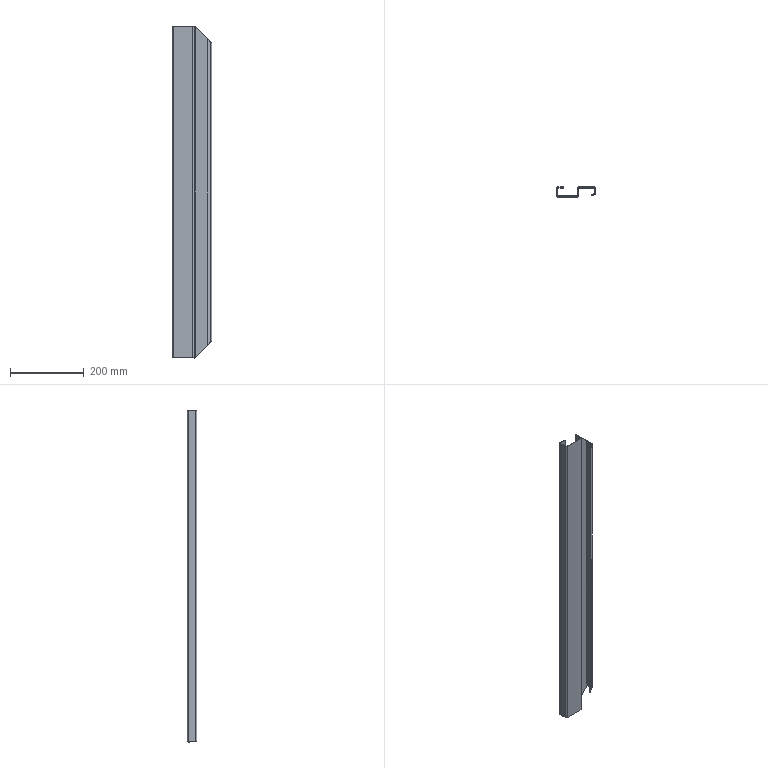Part | STEP file | 750038402 | 1 solid | 32 faces | box 107 x 27 x 900 mm | volume 344520 mm3 | plane 20 | cylinder 12 | commonest cylinder face diameters 4 x6 8 x6
STEP:
#1=CARTESIAN_POINT('',(4.,0.,0.));
#2=VERTEX_POINT('',#1);
#3=CARTESIAN_POINT('',(4.,0.,900.));
#4=VERTEX_POINT('',#3);
#5=CARTESIAN_POINT('',(4.,0.,0.));
#6=DIRECTION('',(0.,0.,1.));
#7=VECTOR('',#6,1000.);
#8=LINE('',#5,#7);
#9=EDGE_CURVE('',#2,#4,#8,.T.);
#10=ORIENTED_EDGE('',*,*,#9,.F.);
#11=CARTESIAN_POINT('',(56.,0.,0.));
#12=VERTEX_POINT('',#11);
#13=CARTESIAN_POINT('',(60.,0.,0.));
#14=DIRECTION('',(-1.,0.,0.));
#15=VECTOR('',#14,1000.);
#16=LINE('',#13,#15);
#17=EDGE_CURVE('',#12,#2,#16,.T.);
#18=ORIENTED_EDGE('',*,*,#17,.F.);
#19=CARTESIAN_POINT('',(56.,0.,900.));
#20=VERTEX_POINT('',#19);
#21=CARTESIAN_POINT('',(56.,0.,0.));
#22=DIRECTION('',(0.,0.,-1.));
#23=VECTOR('',#22,1000.);
#24=LINE('',#21,#23);
#25=EDGE_CURVE('',#20,#12,#24,.T.);
#26=ORIENTED_EDGE('',*,*,#25,.F.);
#27=CARTESIAN_POINT('',(60.,0.,900.));
#28=DIRECTION('',(1.,0.,0.));
#29=VECTOR('',#28,1000.);
#30=LINE('',#27,#29);
#31=EDGE_CURVE('',#4,#20,#30,.T.);
#32=ORIENTED_EDGE('',*,*,#31,.F.);
#33=EDGE_LOOP('',(#10,#18,#26,#32));
#34=FACE_OUTER_BOUND('',#33,.T.);
#35=CARTESIAN_POINT('',(60.,0.,0.));
#36=DIRECTION('',(0.,1.,0.));
#37=DIRECTION('',(0.,0.,1.));
#38=AXIS2_PLACEMENT_3D('',#35,#36,#37);
#39=PLANE('',#38);
#40=ADVANCED_FACE('',(#34),#39,.F.);
#41=CARTESIAN_POINT('',(60.,4.,900.));
#42=VERTEX_POINT('',#41);
#43=CARTESIAN_POINT('',(56.,4.,900.));
#44=DIRECTION('',(0.,0.,1.));
#45=DIRECTION('',(1.,0.,0.));
#46=AXIS2_PLACEMENT_3D('',#43,#44,#45);
#47=CIRCLE('',#46,4.);
#48=EDGE_CURVE('',#20,#42,#47,.T.);
#49=ORIENTED_EDGE('',*,*,#48,.T.);
#50=CARTESIAN_POINT('',(60.,23.,900.));
#51=VERTEX_POINT('',#50);
#52=CARTESIAN_POINT('',(60.,10.535,900.));
#53=DIRECTION('',(0.,1.,0.));
#54=VECTOR('',#53,1000.);
#55=LINE('',#52,#54);
#56=EDGE_CURVE('',#42,#51,#55,.T.);
#57=ORIENTED_EDGE('',*,*,#56,.T.);
#58=CARTESIAN_POINT('',(60.,26.464,900.));
#59=VERTEX_POINT('',#58);
#60=CARTESIAN_POINT('',(60.,10.535,900.));
#61=DIRECTION('',(0.,1.,0.));
#62=VECTOR('',#61,1000.);
#63=LINE('',#60,#62);
#64=EDGE_CURVE('',#51,#59,#63,.T.);
#65=ORIENTED_EDGE('',*,*,#64,.T.);
#66=CARTESIAN_POINT('',(58.,23.,900.));
#67=VERTEX_POINT('',#66);
#68=CARTESIAN_POINT('',(62.,23.,900.));
#69=DIRECTION('',(0.,0.,1.));
#70=DIRECTION('',(1.,0.,0.));
#71=AXIS2_PLACEMENT_3D('',#68,#69,#70);
#72=CIRCLE('',#71,4.);
#73=EDGE_CURVE('',#59,#67,#72,.T.);
#74=ORIENTED_EDGE('',*,*,#73,.T.);
#75=CARTESIAN_POINT('',(58.,4.,900.));
#76=VERTEX_POINT('',#75);
#77=CARTESIAN_POINT('',(58.,10.535,900.));
#78=DIRECTION('',(0.,-1.,0.));
#79=VECTOR('',#78,1000.);
#80=LINE('',#77,#79);
#81=EDGE_CURVE('',#67,#76,#80,.T.);
#82=ORIENTED_EDGE('',*,*,#81,.T.);
#83=CARTESIAN_POINT('',(56.,2.,900.));
#84=VERTEX_POINT('',#83);
#85=CARTESIAN_POINT('',(56.,4.,900.));
#86=DIRECTION('',(0.,0.,-1.));
#87=DIRECTION('',(1.,0.,0.));
#88=AXIS2_PLACEMENT_3D('',#85,#86,#87);
#89=CIRCLE('',#88,2.);
#90=EDGE_CURVE('',#76,#84,#89,.T.);
#91=ORIENTED_EDGE('',*,*,#90,.T.);
#92=CARTESIAN_POINT('',(4.,2.,900.));
#93=VERTEX_POINT('',#92);
#94=CARTESIAN_POINT('',(103.,2.,900.));
#95=DIRECTION('',(-1.,0.,0.));
#96=VECTOR('',#95,1000.);
#97=LINE('',#94,#96);
#98=EDGE_CURVE('',#84,#93,#97,.T.);
#99=ORIENTED_EDGE('',*,*,#98,.T.);
#100=CARTESIAN_POINT('',(2.,4.,900.));
#101=VERTEX_POINT('',#100);
#102=CARTESIAN_POINT('',(4.,4.,900.));
#103=DIRECTION('',(0.,0.,-1.));
#104=DIRECTION('',(1.,0.,0.));
#105=AXIS2_PLACEMENT_3D('',#102,#103,#104);
#106=CIRCLE('',#105,2.);
#107=EDGE_CURVE('',#93,#101,#106,.T.);
#108=ORIENTED_EDGE('',*,*,#107,.T.);
#109=CARTESIAN_POINT('',(2.,23.,900.));
#110=VERTEX_POINT('',#109);
#111=CARTESIAN_POINT('',(2.,10.535,900.));
#112=DIRECTION('',(0.,1.,0.));
#113=VECTOR('',#112,1000.);
#114=LINE('',#111,#113);
#115=EDGE_CURVE('',#101,#110,#114,.T.);
#116=ORIENTED_EDGE('',*,*,#115,.T.);
#117=CARTESIAN_POINT('',(4.,25.,900.));
#118=VERTEX_POINT('',#117);
#119=CARTESIAN_POINT('',(4.,23.,900.));
#120=DIRECTION('',(0.,0.,-1.));
#121=DIRECTION('',(1.,0.,0.));
#122=AXIS2_PLACEMENT_3D('',#119,#120,#121);
#123=CIRCLE('',#122,2.);
#124=EDGE_CURVE('',#110,#118,#123,.T.);
#125=ORIENTED_EDGE('',*,*,#124,.T.);
#126=CARTESIAN_POINT('',(20.,25.,900.));
#127=VERTEX_POINT('',#126);
#128=CARTESIAN_POINT('',(103.,25.,900.));
#129=DIRECTION('',(1.,0.,0.));
#130=VECTOR('',#129,1000.);
#131=LINE('',#128,#130);
#132=EDGE_CURVE('',#118,#127,#131,.T.);
#133=ORIENTED_EDGE('',*,*,#132,.T.);
#134=CARTESIAN_POINT('',(20.,27.,900.));
#135=VERTEX_POINT('',#134);
#136=CARTESIAN_POINT('',(20.,10.535,900.));
#137=DIRECTION('',(0.,1.,0.));
#138=VECTOR('',#137,1000.);
#139=LINE('',#136,#138);
#140=EDGE_CURVE('',#127,#135,#139,.T.);
#141=ORIENTED_EDGE('',*,*,#140,.T.);
#142=CARTESIAN_POINT('',(4.,27.,900.));
#143=VERTEX_POINT('',#142);
#144=CARTESIAN_POINT('',(103.,27.,900.));
#145=DIRECTION('',(-1.,0.,0.));
#146=VECTOR('',#145,1000.);
#147=LINE('',#144,#146);
#148=EDGE_CURVE('',#135,#143,#147,.T.);
#149=ORIENTED_EDGE('',*,*,#148,.T.);
#150=CARTESIAN_POINT('',(0.,23.,900.));
#151=VERTEX_POINT('',#150);
#152=CARTESIAN_POINT('',(4.,23.,900.));
#153=DIRECTION('',(0.,0.,1.));
#154=DIRECTION('',(1.,0.,0.));
#155=AXIS2_PLACEMENT_3D('',#152,#153,#154);
#156=CIRCLE('',#155,4.);
#157=EDGE_CURVE('',#143,#151,#156,.T.);
#158=ORIENTED_EDGE('',*,*,#157,.T.);
#159=CARTESIAN_POINT('',(0.,4.,900.));
#160=VERTEX_POINT('',#159);
#161=CARTESIAN_POINT('',(0.,10.535,900.));
#162=DIRECTION('',(0.,-1.,0.));
#163=VECTOR('',#162,1000.);
#164=LINE('',#161,#163);
#165=EDGE_CURVE('',#151,#160,#164,.T.);
#166=ORIENTED_EDGE('',*,*,#165,.T.);
#167=CARTESIAN_POINT('',(4.,4.,900.));
#168=DIRECTION('',(0.,0.,1.));
#169=DIRECTION('',(1.,0.,0.));
#170=AXIS2_PLACEMENT_3D('',#167,#168,#169);
#171=CIRCLE('',#170,4.);
#172=EDGE_CURVE('',#160,#4,#171,.T.);
#173=ORIENTED_EDGE('',*,*,#172,.T.);
#174=ORIENTED_EDGE('',*,*,#31,.T.);
#175=EDGE_LOOP('',(#49,#57,#65,#74,#82,#91,#99,#108,#116,#125,#133,#141,#149,#158,#166,#173,#174));
#176=FACE_OUTER_BOUND('',#175,.T.);
#177=CARTESIAN_POINT('',(103.,10.535,900.));
#178=DIRECTION('',(0.,0.,1.));
#179=DIRECTION('',(1.,0.,0.));
#180=AXIS2_PLACEMENT_3D('',#177,#178,#179);
#181=PLANE('',#180);
#182=ADVANCED_FACE('',(#176),#181,.T.);
#183=CARTESIAN_POINT('',(0.,4.,0.));
#184=VERTEX_POINT('',#183);
#185=CARTESIAN_POINT('',(4.,4.,0.));
#186=DIRECTION('',(0.,0.,1.));
#187=DIRECTION('',(1.,0.,0.));
#188=AXIS2_PLACEMENT_3D('',#185,#186,#187);
#189=CIRCLE('',#188,4.);
#190=EDGE_CURVE('',#184,#2,#189,.T.);
#191=ORIENTED_EDGE('',*,*,#190,.T.);
#192=ORIENTED_EDGE('',*,*,#9,.T.);
#193=ORIENTED_EDGE('',*,*,#172,.F.);
#194=CARTESIAN_POINT('',(0.,4.,0.));
#195=DIRECTION('',(0.,0.,-1.));
#196=VECTOR('',#195,1000.);
#197=LINE('',#194,#196);
#198=EDGE_CURVE('',#160,#184,#197,.T.);
#199=ORIENTED_EDGE('',*,*,#198,.T.);
#200=EDGE_LOOP('',(#191,#192,#193,#199));
#201=FACE_OUTER_BOUND('',#200,.T.);
#202=CARTESIAN_POINT('',(4.,4.,0.));
#203=DIRECTION('',(0.,0.,1.));
#204=DIRECTION('',(1.,0.,0.));
#205=AXIS2_PLACEMENT_3D('',#202,#203,#204);
#206=CYLINDRICAL_SURFACE('',#205,4.);
#207=ADVANCED_FACE('',(#201),#206,.T.);
#208=CARTESIAN_POINT('',(56.,2.,0.));
#209=VERTEX_POINT('',#208);
#210=CARTESIAN_POINT('',(58.,4.,0.));
#211=VERTEX_POINT('',#210);
#212=CARTESIAN_POINT('',(56.,4.,0.));
#213=DIRECTION('',(0.,0.,1.));
#214=DIRECTION('',(1.,0.,0.));
#215=AXIS2_PLACEMENT_3D('',#212,#213,#214);
#216=CIRCLE('',#215,2.);
#217=EDGE_CURVE('',#209,#211,#216,.T.);
#218=ORIENTED_EDGE('',*,*,#217,.T.);
#219=CARTESIAN_POINT('',(58.,23.,0.));
#220=VERTEX_POINT('',#219);
#221=CARTESIAN_POINT('',(58.,6.153,0.));
#222=DIRECTION('',(0.,1.,0.));
#223=VECTOR('',#222,1000.);
#224=LINE('',#221,#223);
#225=EDGE_CURVE('',#211,#220,#224,.T.);
#226=ORIENTED_EDGE('',*,*,#225,.T.);
#227=CARTESIAN_POINT('',(60.,26.464,0.));
#228=VERTEX_POINT('',#227);
#229=CARTESIAN_POINT('',(62.,23.,0.));
#230=DIRECTION('',(0.,0.,-1.));
#231=DIRECTION('',(1.,0.,0.));
#232=AXIS2_PLACEMENT_3D('',#229,#230,#231);
#233=CIRCLE('',#232,4.);
#234=EDGE_CURVE('',#220,#228,#233,.T.);
#235=ORIENTED_EDGE('',*,*,#234,.T.);
#236=CARTESIAN_POINT('',(60.,23.,0.));
#237=VERTEX_POINT('',#236);
#238=CARTESIAN_POINT('',(60.,6.153,0.));
#239=DIRECTION('',(0.,-1.,0.));
#240=VECTOR('',#239,1000.);
#241=LINE('',#238,#240);
#242=EDGE_CURVE('',#228,#237,#241,.T.);
#243=ORIENTED_EDGE('',*,*,#242,.T.);
#244=CARTESIAN_POINT('',(60.,4.,0.));
#245=VERTEX_POINT('',#244);
#246=CARTESIAN_POINT('',(60.,6.153,0.));
#247=DIRECTION('',(0.,-1.,0.));
#248=VECTOR('',#247,1000.);
#249=LINE('',#246,#248);
#250=EDGE_CURVE('',#237,#245,#249,.T.);
#251=ORIENTED_EDGE('',*,*,#250,.T.);
#252=CARTESIAN_POINT('',(56.,4.,0.));
#253=DIRECTION('',(0.,0.,-1.));
#254=DIRECTION('',(1.,0.,0.));
#255=AXIS2_PLACEMENT_3D('',#252,#253,#254);
#256=CIRCLE('',#255,4.);
#257=EDGE_CURVE('',#245,#12,#256,.T.);
#258=ORIENTED_EDGE('',*,*,#257,.T.);
#259=ORIENTED_EDGE('',*,*,#17,.T.);
#260=ORIENTED_EDGE('',*,*,#190,.F.);
#261=CARTESIAN_POINT('',(0.,23.,0.));
#262=VERTEX_POINT('',#261);
#263=CARTESIAN_POINT('',(0.,6.153,0.));
#264=DIRECTION('',(0.,1.,0.));
#265=VECTOR('',#264,1000.);
#266=LINE('',#263,#265);
#267=EDGE_CURVE('',#184,#262,#266,.T.);
#268=ORIENTED_EDGE('',*,*,#267,.T.);
#269=CARTESIAN_POINT('',(4.,27.,0.));
#270=VERTEX_POINT('',#269);
#271=CARTESIAN_POINT('',(4.,23.,0.));
#272=DIRECTION('',(0.,0.,-1.));
#273=DIRECTION('',(1.,0.,0.));
#274=AXIS2_PLACEMENT_3D('',#271,#272,#273);
#275=CIRCLE('',#274,4.);
#276=EDGE_CURVE('',#262,#270,#275,.T.);
#277=ORIENTED_EDGE('',*,*,#276,.T.);
#278=CARTESIAN_POINT('',(20.,27.,0.));
#279=VERTEX_POINT('',#278);
#280=CARTESIAN_POINT('',(94.375,27.,0.));
#281=DIRECTION('',(1.,0.,0.));
#282=VECTOR('',#281,1000.);
#283=LINE('',#280,#282);
#284=EDGE_CURVE('',#270,#279,#283,.T.);
#285=ORIENTED_EDGE('',*,*,#284,.T.);
#286=CARTESIAN_POINT('',(20.,25.,0.));
#287=VERTEX_POINT('',#286);
#288=CARTESIAN_POINT('',(20.,6.153,0.));
#289=DIRECTION('',(0.,-1.,0.));
#290=VECTOR('',#289,1000.);
#291=LINE('',#288,#290);
#292=EDGE_CURVE('',#279,#287,#291,.T.);
#293=ORIENTED_EDGE('',*,*,#292,.T.);
#294=CARTESIAN_POINT('',(4.,25.,0.));
#295=VERTEX_POINT('',#294);
#296=CARTESIAN_POINT('',(94.375,25.,0.));
#297=DIRECTION('',(-1.,0.,0.));
#298=VECTOR('',#297,1000.);
#299=LINE('',#296,#298);
#300=EDGE_CURVE('',#287,#295,#299,.T.);
#301=ORIENTED_EDGE('',*,*,#300,.T.);
#302=CARTESIAN_POINT('',(2.,23.,0.));
#303=VERTEX_POINT('',#302);
#304=CARTESIAN_POINT('',(4.,23.,0.));
#305=DIRECTION('',(0.,0.,1.));
#306=DIRECTION('',(1.,0.,0.));
#307=AXIS2_PLACEMENT_3D('',#304,#305,#306);
#308=CIRCLE('',#307,2.);
#309=EDGE_CURVE('',#295,#303,#308,.T.);
#310=ORIENTED_EDGE('',*,*,#309,.T.);
#311=CARTESIAN_POINT('',(2.,4.,0.));
#312=VERTEX_POINT('',#311);
#313=CARTESIAN_POINT('',(2.,6.153,0.));
#314=DIRECTION('',(0.,-1.,0.));
#315=VECTOR('',#314,1000.);
#316=LINE('',#313,#315);
#317=EDGE_CURVE('',#303,#312,#316,.T.);
#318=ORIENTED_EDGE('',*,*,#317,.T.);
#319=CARTESIAN_POINT('',(4.,2.,0.));
#320=VERTEX_POINT('',#319);
#321=CARTESIAN_POINT('',(4.,4.,0.));
#322=DIRECTION('',(0.,0.,1.));
#323=DIRECTION('',(1.,0.,0.));
#324=AXIS2_PLACEMENT_3D('',#321,#322,#323);
#325=CIRCLE('',#324,2.);
#326=EDGE_CURVE('',#312,#320,#325,.T.);
#327=ORIENTED_EDGE('',*,*,#326,.T.);
#328=CARTESIAN_POINT('',(94.375,2.,0.));
#329=DIRECTION('',(1.,0.,0.));
#330=VECTOR('',#329,1000.);
#331=LINE('',#328,#330);
#332=EDGE_CURVE('',#320,#209,#331,.T.);
#333=ORIENTED_EDGE('',*,*,#332,.T.);
#334=EDGE_LOOP('',(#218,#226,#235,#243,#251,#258,#259,#260,#268,#277,#285,#293,#301,#310,#318,#327,#333));
#335=FACE_OUTER_BOUND('',#334,.T.);
#336=CARTESIAN_POINT('',(94.375,6.153,0.));
#337=DIRECTION('',(0.,0.,-1.));
#338=DIRECTION('',(-1.,0.,0.));
#339=AXIS2_PLACEMENT_3D('',#336,#337,#338);
#340=PLANE('',#339);
#341=ADVANCED_FACE('',(#335),#340,.T.);
#342=ORIENTED_EDGE('',*,*,#257,.F.);
#343=CARTESIAN_POINT('',(60.,4.,0.));
#344=DIRECTION('',(0.,0.,1.));
#345=VECTOR('',#344,1000.);
#346=LINE('',#343,#345);
#347=EDGE_CURVE('',#245,#42,#346,.T.);
#348=ORIENTED_EDGE('',*,*,#347,.T.);
#349=ORIENTED_EDGE('',*,*,#48,.F.);
#350=ORIENTED_EDGE('',*,*,#25,.T.);
#351=EDGE_LOOP('',(#342,#348,#349,#350));
#352=FACE_OUTER_BOUND('',#351,.T.);
#353=CARTESIAN_POINT('',(56.,4.,0.));
#354=DIRECTION('',(0.,0.,1.));
#355=DIRECTION('',(1.,0.,0.));
#356=AXIS2_PLACEMENT_3D('',#353,#354,#355);
#357=CYLINDRICAL_SURFACE('',#356,4.);
#358=ADVANCED_FACE('',(#352),#357,.T.);
#359=ORIENTED_EDGE('',*,*,#347,.F.);
#360=ORIENTED_EDGE('',*,*,#250,.F.);
#361=CARTESIAN_POINT('',(60.,23.,0.));
#362=DIRECTION('',(0.,0.,-1.));
#363=VECTOR('',#362,1000.);
#364=LINE('',#361,#363);
#365=EDGE_CURVE('',#51,#237,#364,.T.);
#366=ORIENTED_EDGE('',*,*,#365,.F.);
#367=ORIENTED_EDGE('',*,*,#56,.F.);
#368=EDGE_LOOP('',(#359,#360,#366,#367));
#369=FACE_OUTER_BOUND('',#368,.T.);
#370=CARTESIAN_POINT('',(60.,25.,0.));
#371=DIRECTION('',(-1.,0.,0.));
#372=DIRECTION('',(0.,0.,1.));
#373=AXIS2_PLACEMENT_3D('',#370,#371,#372);
#374=PLANE('',#373);
#375=ADVANCED_FACE('',(#369),#374,.F.);
#376=CARTESIAN_POINT('',(0.,23.,0.));
#377=DIRECTION('',(0.,0.,1.));
#378=VECTOR('',#377,1000.);
#379=LINE('',#376,#378);
#380=EDGE_CURVE('',#262,#151,#379,.T.);
#381=ORIENTED_EDGE('',*,*,#380,.F.);
#382=ORIENTED_EDGE('',*,*,#267,.F.);
#383=ORIENTED_EDGE('',*,*,#198,.F.);
#384=ORIENTED_EDGE('',*,*,#165,.F.);
#385=EDGE_LOOP('',(#381,#382,#383,#384));
#386=FACE_OUTER_BOUND('',#385,.T.);
#387=CARTESIAN_POINT('',(0.,0.,0.));
#388=DIRECTION('',(1.,0.,0.));
#389=DIRECTION('',(0.,0.,-1.));
#390=AXIS2_PLACEMENT_3D('',#387,#388,#389);
#391=PLANE('',#390);
#392=ADVANCED_FACE('',(#386),#391,.F.);
#393=ORIENTED_EDGE('',*,*,#276,.F.);
#394=ORIENTED_EDGE('',*,*,#380,.T.);
#395=ORIENTED_EDGE('',*,*,#157,.F.);
#396=CARTESIAN_POINT('',(4.,27.,0.));
#397=DIRECTION('',(0.,0.,-1.));
#398=VECTOR('',#397,1000.);
#399=LINE('',#396,#398);
#400=EDGE_CURVE('',#143,#270,#399,.T.);
#401=ORIENTED_EDGE('',*,*,#400,.T.);
#402=EDGE_LOOP('',(#393,#394,#395,#401));
#403=FACE_OUTER_BOUND('',#402,.T.);
#404=CARTESIAN_POINT('',(4.,23.,0.));
#405=DIRECTION('',(0.,0.,1.));
#406=DIRECTION('',(1.,0.,0.));
#407=AXIS2_PLACEMENT_3D('',#404,#405,#406);
#408=CYLINDRICAL_SURFACE('',#407,4.);
#409=ADVANCED_FACE('',(#403),#408,.T.);
#410=CARTESIAN_POINT('',(20.,27.,0.));
#411=DIRECTION('',(0.,0.,1.));
#412=VECTOR('',#411,1000.);
#413=LINE('',#410,#412);
#414=EDGE_CURVE('',#279,#135,#413,.T.);
#415=ORIENTED_EDGE('',*,*,#414,.F.);
#416=ORIENTED_EDGE('',*,*,#284,.F.);
#417=ORIENTED_EDGE('',*,*,#400,.F.);
#418=ORIENTED_EDGE('',*,*,#148,.F.);
#419=EDGE_LOOP('',(#415,#416,#417,#418));
#420=FACE_OUTER_BOUND('',#419,.T.);
#421=CARTESIAN_POINT('',(0.,27.,0.));
#422=DIRECTION('',(0.,-1.,0.));
#423=DIRECTION('',(0.,0.,-1.));
#424=AXIS2_PLACEMENT_3D('',#421,#422,#423);
#425=PLANE('',#424);
#426=ADVANCED_FACE('',(#420),#425,.F.);
#427=ORIENTED_EDGE('',*,*,#292,.F.);
#428=ORIENTED_EDGE('',*,*,#414,.T.);
#429=ORIENTED_EDGE('',*,*,#140,.F.);
#430=CARTESIAN_POINT('',(20.,25.,0.));
#431=DIRECTION('',(0.,0.,-1.));
#432=VECTOR('',#431,1000.);
#433=LINE('',#430,#432);
#434=EDGE_CURVE('',#127,#287,#433,.T.);
#435=ORIENTED_EDGE('',*,*,#434,.T.);
#436=EDGE_LOOP('',(#427,#428,#429,#435));
#437=FACE_OUTER_BOUND('',#436,.T.);
#438=CARTESIAN_POINT('',(20.,27.,0.));
#439=DIRECTION('',(1.,0.,0.));
#440=DIRECTION('',(0.,0.,-1.));
#441=AXIS2_PLACEMENT_3D('',#438,#439,#440);
#442=PLANE('',#441);
#443=ADVANCED_FACE('',(#437),#442,.T.);
#444=ORIENTED_EDGE('',*,*,#300,.F.);
#445=ORIENTED_EDGE('',*,*,#434,.F.);
#446=ORIENTED_EDGE('',*,*,#132,.F.);
#447=CARTESIAN_POINT('',(4.,25.,0.));
#448=DIRECTION('',(0.,0.,-1.));
#449=VECTOR('',#448,1000.);
#450=LINE('',#447,#449);
#451=EDGE_CURVE('',#118,#295,#450,.T.);
#452=ORIENTED_EDGE('',*,*,#451,.T.);
#453=EDGE_LOOP('',(#444,#445,#446,#452));
#454=FACE_OUTER_BOUND('',#453,.T.);
#455=CARTESIAN_POINT('',(0.,25.,0.));
#456=DIRECTION('',(0.,-1.,0.));
#457=DIRECTION('',(0.,0.,-1.));
#458=AXIS2_PLACEMENT_3D('',#455,#456,#457);
#459=PLANE('',#458);
#460=ADVANCED_FACE('',(#454),#459,.T.);
#461=CARTESIAN_POINT('',(2.,23.,0.));
#462=DIRECTION('',(0.,0.,1.));
#463=VECTOR('',#462,1000.);
#464=LINE('',#461,#463);
#465=EDGE_CURVE('',#303,#110,#464,.T.);
#466=ORIENTED_EDGE('',*,*,#465,.F.);
#467=ORIENTED_EDGE('',*,*,#309,.F.);
#468=ORIENTED_EDGE('',*,*,#451,.F.);
#469=ORIENTED_EDGE('',*,*,#124,.F.);
#470=EDGE_LOOP('',(#466,#467,#468,#469));
#471=FACE_OUTER_BOUND('',#470,.T.);
#472=CARTESIAN_POINT('',(4.,23.,0.));
#473=DIRECTION('',(0.,0.,1.));
#474=DIRECTION('',(1.,0.,0.));
#475=AXIS2_PLACEMENT_3D('',#472,#473,#474);
#476=CYLINDRICAL_SURFACE('',#475,2.);
#477=ADVANCED_FACE('',(#471),#476,.F.);
#478=ORIENTED_EDGE('',*,*,#317,.F.);
#479=ORIENTED_EDGE('',*,*,#465,.T.);
#480=ORIENTED_EDGE('',*,*,#115,.F.);
#481=CARTESIAN_POINT('',(2.,4.,0.));
#482=DIRECTION('',(0.,0.,-1.));
#483=VECTOR('',#482,1000.);
#484=LINE('',#481,#483);
#485=EDGE_CURVE('',#101,#312,#484,.T.);
#486=ORIENTED_EDGE('',*,*,#485,.T.);
#487=EDGE_LOOP('',(#478,#479,#480,#486));
#488=FACE_OUTER_BOUND('',#487,.T.);
#489=CARTESIAN_POINT('',(2.,0.,0.));
#490=DIRECTION('',(1.,0.,0.));
#491=DIRECTION('',(0.,0.,-1.));
#492=AXIS2_PLACEMENT_3D('',#489,#490,#491);
#493=PLANE('',#492);
#494=ADVANCED_FACE('',(#488),#493,.T.);
#495=CARTESIAN_POINT('',(4.,2.,0.));
#496=DIRECTION('',(0.,0.,1.));
#497=VECTOR('',#496,1000.);
#498=LINE('',#495,#497);
#499=EDGE_CURVE('',#320,#93,#498,.T.);
#500=ORIENTED_EDGE('',*,*,#499,.F.);
#501=ORIENTED_EDGE('',*,*,#326,.F.);
#502=ORIENTED_EDGE('',*,*,#485,.F.);
#503=ORIENTED_EDGE('',*,*,#107,.F.);
#504=EDGE_LOOP('',(#500,#501,#502,#503));
#505=FACE_OUTER_BOUND('',#504,.T.);
#506=CARTESIAN_POINT('',(4.,4.,0.));
#507=DIRECTION('',(0.,0.,1.));
#508=DIRECTION('',(1.,0.,0.));
#509=AXIS2_PLACEMENT_3D('',#506,#507,#508);
#510=CYLINDRICAL_SURFACE('',#509,2.);
#511=ADVANCED_FACE('',(#505),#510,.F.);
#512=ORIENTED_EDGE('',*,*,#332,.F.);
#513=ORIENTED_EDGE('',*,*,#499,.T.);
#514=ORIENTED_EDGE('',*,*,#98,.F.);
#515=CARTESIAN_POINT('',(56.,2.,0.));
#516=DIRECTION('',(0.,0.,-1.));
#517=VECTOR('',#516,1000.);
#518=LINE('',#515,#517);
#519=EDGE_CURVE('',#84,#209,#518,.T.);
#520=ORIENTED_EDGE('',*,*,#519,.T.);
#521=EDGE_LOOP('',(#512,#513,#514,#520));
#522=FACE_OUTER_BOUND('',#521,.T.);
#523=CARTESIAN_POINT('',(60.,2.,0.));
#524=DIRECTION('',(0.,1.,0.));
#525=DIRECTION('',(0.,0.,1.));
#526=AXIS2_PLACEMENT_3D('',#523,#524,#525);
#527=PLANE('',#526);
#528=ADVANCED_FACE('',(#522),#527,.T.);
#529=CARTESIAN_POINT('',(58.,4.,0.));
#530=DIRECTION('',(0.,0.,1.));
#531=VECTOR('',#530,1000.);
#532=LINE('',#529,#531);
#533=EDGE_CURVE('',#211,#76,#532,.T.);
#534=ORIENTED_EDGE('',*,*,#533,.F.);
#535=ORIENTED_EDGE('',*,*,#217,.F.);
#536=ORIENTED_EDGE('',*,*,#519,.F.);
#537=ORIENTED_EDGE('',*,*,#90,.F.);
#538=EDGE_LOOP('',(#534,#535,#536,#537));
#539=FACE_OUTER_BOUND('',#538,.T.);
#540=CARTESIAN_POINT('',(56.,4.,0.));
#541=DIRECTION('',(0.,0.,1.));
#542=DIRECTION('',(1.,0.,0.));
#543=AXIS2_PLACEMENT_3D('',#540,#541,#542);
#544=CYLINDRICAL_SURFACE('',#543,2.);
#545=ADVANCED_FACE('',(#539),#544,.F.);
#546=ORIENTED_EDGE('',*,*,#225,.F.);
#547=ORIENTED_EDGE('',*,*,#533,.T.);
#548=ORIENTED_EDGE('',*,*,#81,.F.);
#549=CARTESIAN_POINT('',(58.,23.,0.));
#550=DIRECTION('',(0.,0.,-1.));
#551=VECTOR('',#550,1000.);
#552=LINE('',#549,#551);
#553=EDGE_CURVE('',#67,#220,#552,.T.);
#554=ORIENTED_EDGE('',*,*,#553,.T.);
#555=EDGE_LOOP('',(#546,#547,#548,#554));
#556=FACE_OUTER_BOUND('',#555,.T.);
#557=CARTESIAN_POINT('',(58.,25.,0.));
#558=DIRECTION('',(-1.,0.,0.));
#559=DIRECTION('',(0.,0.,1.));
#560=AXIS2_PLACEMENT_3D('',#557,#558,#559);
#561=PLANE('',#560);
#562=ADVANCED_FACE('',(#556),#561,.T.);
#563=CARTESIAN_POINT('',(62.,27.,898.));
#564=VERTEX_POINT('',#563);
#565=CARTESIAN_POINT('',(60.,26.464,900.));
#566=CARTESIAN_POINT('',(60.612,26.817,899.388));
#567=CARTESIAN_POINT('',(61.294,27.,898.706));
#568=CARTESIAN_POINT('',(62.,27.,898.));
#569=(BOUNDED_CURVE()B_SPLINE_CURVE(3,(#565,#566,#567,#568),.UNSPECIFIED.,.F.,.F.)B_SPLINE_CURVE_WITH_KNOTS((4,4),(1.047,1.571),.UNSPECIFIED.)CURVE()GEOMETRIC_REPRESENTATION_ITEM()RATIONAL_B_SPLINE_CURVE((1.,0.9773,0.9773,1.))REPRESENTATION_ITEM(''));
#570=EDGE_CURVE('',#59,#564,#569,.T.);
#571=ORIENTED_EDGE('',*,*,#570,.T.);
#572=CARTESIAN_POINT('',(62.,27.,2.));
#573=VERTEX_POINT('',#572);
#574=CARTESIAN_POINT('',(62.,27.,0.));
#575=DIRECTION('',(0.,0.,-1.));
#576=VECTOR('',#575,1000.);
#577=LINE('',#574,#576);
#578=EDGE_CURVE('',#564,#573,#577,.T.);
#579=ORIENTED_EDGE('',*,*,#578,.T.);
#580=CARTESIAN_POINT('',(62.,27.,2.));
#581=CARTESIAN_POINT('',(61.294,27.,1.294));
#582=CARTESIAN_POINT('',(60.612,26.817,0.6116));
#583=CARTESIAN_POINT('',(60.,26.464,0.));
#584=(BOUNDED_CURVE()B_SPLINE_CURVE(3,(#580,#581,#582,#583),.UNSPECIFIED.,.F.,.F.)B_SPLINE_CURVE_WITH_KNOTS((4,4),(1.571,2.094),.UNSPECIFIED.)CURVE()GEOMETRIC_REPRESENTATION_ITEM()RATIONAL_B_SPLINE_CURVE((1.,0.9773,0.9773,1.))REPRESENTATION_ITEM(''));
#585=EDGE_CURVE('',#573,#228,#584,.T.);
#586=ORIENTED_EDGE('',*,*,#585,.T.);
#587=ORIENTED_EDGE('',*,*,#234,.F.);
#588=ORIENTED_EDGE('',*,*,#553,.F.);
#589=ORIENTED_EDGE('',*,*,#73,.F.);
#590=EDGE_LOOP('',(#571,#579,#586,#587,#588,#589));
#591=FACE_OUTER_BOUND('',#590,.T.);
#592=CARTESIAN_POINT('',(62.,23.,0.));
#593=DIRECTION('',(0.,0.,1.));
#594=DIRECTION('',(1.,0.,0.));
#595=AXIS2_PLACEMENT_3D('',#592,#593,#594);
#596=CYLINDRICAL_SURFACE('',#595,4.);
#597=ADVANCED_FACE('',(#591),#596,.T.);
#598=CARTESIAN_POINT('',(105.,23.,855.));
#599=VERTEX_POINT('',#598);
#600=CARTESIAN_POINT('',(103.,25.,857.));
#601=VERTEX_POINT('',#600);
#602=CARTESIAN_POINT('',(105.,23.,855.));
#603=CARTESIAN_POINT('',(105.,24.172,855.));
#604=CARTESIAN_POINT('',(104.172,25.,855.828));
#605=CARTESIAN_POINT('',(103.,25.,857.));
#606=(BOUNDED_CURVE()B_SPLINE_CURVE(3,(#602,#603,#604,#605),.UNSPECIFIED.,.F.,.F.)B_SPLINE_CURVE_WITH_KNOTS((4,4),(3.142,4.712),.UNSPECIFIED.)CURVE()GEOMETRIC_REPRESENTATION_ITEM()RATIONAL_B_SPLINE_CURVE((1.,0.8047,0.8047,1.))REPRESENTATION_ITEM(''));
#607=EDGE_CURVE('',#599,#601,#606,.T.);
#608=ORIENTED_EDGE('',*,*,#607,.F.);
#609=CARTESIAN_POINT('',(105.,10.535,855.));
#610=VERTEX_POINT('',#609);
#611=CARTESIAN_POINT('',(105.,29.7,855.));
#612=DIRECTION('',(0.,1.,0.));
#613=VECTOR('',#612,1000.);
#614=LINE('',#611,#613);
#615=EDGE_CURVE('',#610,#599,#614,.T.);
#616=ORIENTED_EDGE('',*,*,#615,.F.);
#617=CARTESIAN_POINT('',(103.518,8.603,856.482));
#618=VERTEX_POINT('',#617);
#619=CARTESIAN_POINT('',(103.518,8.603,856.482));
#620=CARTESIAN_POINT('',(104.427,8.846,855.573));
#621=CARTESIAN_POINT('',(105.,9.593,855.));
#622=CARTESIAN_POINT('',(105.,10.535,855.));
#623=(BOUNDED_CURVE()B_SPLINE_CURVE(3,(#619,#620,#621,#622),.UNSPECIFIED.,.F.,.T.)B_SPLINE_CURVE_WITH_KNOTS((4,4),(1.833,3.142),.UNSPECIFIED.)CURVE()GEOMETRIC_REPRESENTATION_ITEM()RATIONAL_B_SPLINE_CURVE((1.,0.8622,0.8622,1.))REPRESENTATION_ITEM(''));
#624=EDGE_CURVE('',#618,#610,#623,.T.);
#625=ORIENTED_EDGE('',*,*,#624,.F.);
#626=CARTESIAN_POINT('',(94.375,6.153,865.625));
#627=VERTEX_POINT('',#626);
#628=CARTESIAN_POINT('',(94.375,6.153,865.625));
#629=DIRECTION('',(0.6947,0.1862,-0.6947));
#630=VECTOR('',#629,1000.);
#631=LINE('',#628,#630);
#632=EDGE_CURVE('',#627,#618,#631,.T.);
#633=ORIENTED_EDGE('',*,*,#632,.F.);
#634=CARTESIAN_POINT('',(94.892,4.221,865.108));
#635=VERTEX_POINT('',#634);
#636=CARTESIAN_POINT('',(94.892,4.221,865.108));
#637=DIRECTION('',(-0.2506,0.9351,0.2506));
#638=VECTOR('',#637,1000.);
#639=LINE('',#636,#638);
#640=EDGE_CURVE('',#635,#627,#639,.T.);
#641=ORIENTED_EDGE('',*,*,#640,.F.);
#642=CARTESIAN_POINT('',(104.035,6.671,855.965));
#643=VERTEX_POINT('',#642);
#644=CARTESIAN_POINT('',(104.035,6.671,855.965));
#645=DIRECTION('',(-0.6947,-0.1862,0.6947));
#646=VECTOR('',#645,1000.);
#647=LINE('',#644,#646);
#648=EDGE_CURVE('',#643,#635,#647,.T.);
#649=ORIENTED_EDGE('',*,*,#648,.F.);
#650=CARTESIAN_POINT('',(107.,10.535,853.));
#651=VERTEX_POINT('',#650);
#652=CARTESIAN_POINT('',(107.,10.535,853.));
#653=CARTESIAN_POINT('',(107.,8.652,853.));
#654=CARTESIAN_POINT('',(105.854,7.158,854.146));
#655=CARTESIAN_POINT('',(104.035,6.671,855.965));
#656=(BOUNDED_CURVE()B_SPLINE_CURVE(3,(#652,#653,#654,#655),.UNSPECIFIED.,.F.,.T.)B_SPLINE_CURVE_WITH_KNOTS((4,4),(3.142,4.451),.UNSPECIFIED.)CURVE()GEOMETRIC_REPRESENTATION_ITEM()RATIONAL_B_SPLINE_CURVE((1.,0.8622,0.8622,1.))REPRESENTATION_ITEM(''));
#657=EDGE_CURVE('',#651,#643,#656,.T.);
#658=ORIENTED_EDGE('',*,*,#657,.F.);
#659=CARTESIAN_POINT('',(107.,23.,853.));
#660=VERTEX_POINT('',#659);
#661=CARTESIAN_POINT('',(107.,29.7,853.));
#662=DIRECTION('',(0.,-1.,0.));
#663=VECTOR('',#662,1000.);
#664=LINE('',#661,#663);
#665=EDGE_CURVE('',#660,#651,#664,.T.);
#666=ORIENTED_EDGE('',*,*,#665,.F.);
#667=CARTESIAN_POINT('',(103.,27.,857.));
#668=VERTEX_POINT('',#667);
#669=CARTESIAN_POINT('',(103.,27.,857.));
#670=CARTESIAN_POINT('',(105.343,27.,854.657));
#671=CARTESIAN_POINT('',(107.,25.343,853.));
#672=CARTESIAN_POINT('',(107.,23.,853.));
#673=(BOUNDED_CURVE()B_SPLINE_CURVE(3,(#669,#670,#671,#672),.UNSPECIFIED.,.F.,.F.)B_SPLINE_CURVE_WITH_KNOTS((4,4),(1.571,3.142),.UNSPECIFIED.)CURVE()GEOMETRIC_REPRESENTATION_ITEM()RATIONAL_B_SPLINE_CURVE((1.,0.8047,0.8047,1.))REPRESENTATION_ITEM(''));
#674=EDGE_CURVE('',#668,#660,#673,.T.);
#675=ORIENTED_EDGE('',*,*,#674,.F.);
#676=CARTESIAN_POINT('',(60.,27.,900.));
#677=DIRECTION('',(0.7071,0.,-0.7071));
#678=VECTOR('',#677,1000.);
#679=LINE('',#676,#678);
#680=EDGE_CURVE('',#564,#668,#679,.T.);
#681=ORIENTED_EDGE('',*,*,#680,.F.);
#682=ORIENTED_EDGE('',*,*,#570,.F.);
#683=ORIENTED_EDGE('',*,*,#64,.F.);
#684=CARTESIAN_POINT('',(62.,25.,898.));
#685=VERTEX_POINT('',#684);
#686=CARTESIAN_POINT('',(62.,25.,898.));
#687=CARTESIAN_POINT('',(60.828,25.,899.172));
#688=CARTESIAN_POINT('',(60.,24.172,900.));
#689=CARTESIAN_POINT('',(60.,23.,900.));
#690=(BOUNDED_CURVE()B_SPLINE_CURVE(3,(#686,#687,#688,#689),.UNSPECIFIED.,.F.,.T.)B_SPLINE_CURVE_WITH_KNOTS((4,4),(4.712,6.283),.UNSPECIFIED.)CURVE()GEOMETRIC_REPRESENTATION_ITEM()RATIONAL_B_SPLINE_CURVE((1.,0.8047,0.8047,1.))REPRESENTATION_ITEM(''));
#691=EDGE_CURVE('',#685,#51,#690,.T.);
#692=ORIENTED_EDGE('',*,*,#691,.F.);
#693=CARTESIAN_POINT('',(60.,25.,900.));
#694=DIRECTION('',(-0.7071,0.,0.7071));
#695=VECTOR('',#694,1000.);
#696=LINE('',#693,#695);
#697=EDGE_CURVE('',#601,#685,#696,.T.);
#698=ORIENTED_EDGE('',*,*,#697,.F.);
#699=EDGE_LOOP('',(#608,#616,#625,#633,#641,#649,#658,#666,#675,#681,#682,#683,#692,#698));
#700=FACE_OUTER_BOUND('',#699,.T.);
#701=CARTESIAN_POINT('',(60.,29.7,900.));
#702=DIRECTION('',(-0.7071,0.,-0.7071));
#703=DIRECTION('',(-0.7071,0.,0.7071));
#704=AXIS2_PLACEMENT_3D('',#701,#702,#703);
#705=PLANE('',#704);
#706=ADVANCED_FACE('',(#700),#705,.F.);
#707=ORIENTED_EDGE('',*,*,#585,.F.);
#708=CARTESIAN_POINT('',(103.,27.,43.));
#709=VERTEX_POINT('',#708);
#710=CARTESIAN_POINT('',(107.376,27.,47.376));
#711=DIRECTION('',(-0.7071,0.,-0.7071));
#712=VECTOR('',#711,1000.);
#713=LINE('',#710,#712);
#714=EDGE_CURVE('',#709,#573,#713,.T.);
#715=ORIENTED_EDGE('',*,*,#714,.F.);
#716=CARTESIAN_POINT('',(107.,23.,47.));
#717=VERTEX_POINT('',#716);
#718=CARTESIAN_POINT('',(107.,23.,47.));
#719=CARTESIAN_POINT('',(107.,25.343,47.));
#720=CARTESIAN_POINT('',(105.343,27.,45.343));
#721=CARTESIAN_POINT('',(103.,27.,43.));
#722=(BOUNDED_CURVE()B_SPLINE_CURVE(3,(#718,#719,#720,#721),.UNSPECIFIED.,.F.,.F.)B_SPLINE_CURVE_WITH_KNOTS((4,4),(0.,1.571),.UNSPECIFIED.)CURVE()GEOMETRIC_REPRESENTATION_ITEM()RATIONAL_B_SPLINE_CURVE((1.,0.8047,0.8047,1.))REPRESENTATION_ITEM(''));
#723=EDGE_CURVE('',#717,#709,#722,.T.);
#724=ORIENTED_EDGE('',*,*,#723,.F.);
#725=CARTESIAN_POINT('',(107.,10.535,47.));
#726=VERTEX_POINT('',#725);
#727=CARTESIAN_POINT('',(107.,29.7,47.));
#728=DIRECTION('',(0.,1.,0.));
#729=VECTOR('',#728,1000.);
#730=LINE('',#727,#729);
#731=EDGE_CURVE('',#726,#717,#730,.T.);
#732=ORIENTED_EDGE('',*,*,#731,.F.);
#733=CARTESIAN_POINT('',(104.035,6.671,44.035));
#734=VERTEX_POINT('',#733);
#735=CARTESIAN_POINT('',(104.035,6.671,44.035));
#736=CARTESIAN_POINT('',(105.854,7.158,45.854));
#737=CARTESIAN_POINT('',(107.,8.652,47.));
#738=CARTESIAN_POINT('',(107.,10.535,47.));
#739=(BOUNDED_CURVE()B_SPLINE_CURVE(3,(#735,#736,#737,#738),.UNSPECIFIED.,.F.,.T.)B_SPLINE_CURVE_WITH_KNOTS((4,4),(4.974,6.283),.UNSPECIFIED.)CURVE()GEOMETRIC_REPRESENTATION_ITEM()RATIONAL_B_SPLINE_CURVE((1.,0.8622,0.8622,1.))REPRESENTATION_ITEM(''));
#740=EDGE_CURVE('',#734,#726,#739,.T.);
#741=ORIENTED_EDGE('',*,*,#740,.F.);
#742=CARTESIAN_POINT('',(94.892,4.221,34.892));
#743=VERTEX_POINT('',#742);
#744=CARTESIAN_POINT('',(94.892,4.221,34.892));
#745=DIRECTION('',(0.6947,0.1862,0.6947));
#746=VECTOR('',#745,1000.);
#747=LINE('',#744,#746);
#748=EDGE_CURVE('',#743,#734,#747,.T.);
#749=ORIENTED_EDGE('',*,*,#748,.F.);
#750=CARTESIAN_POINT('',(94.375,6.153,34.375));
#751=VERTEX_POINT('',#750);
#752=CARTESIAN_POINT('',(94.375,6.153,34.375));
#753=DIRECTION('',(0.2506,-0.9351,0.2506));
#754=VECTOR('',#753,1000.);
#755=LINE('',#752,#754);
#756=EDGE_CURVE('',#751,#743,#755,.T.);
#757=ORIENTED_EDGE('',*,*,#756,.F.);
#758=CARTESIAN_POINT('',(103.518,8.603,43.518));
#759=VERTEX_POINT('',#758);
#760=CARTESIAN_POINT('',(103.518,8.603,43.518));
#761=DIRECTION('',(-0.6947,-0.1862,-0.6947));
#762=VECTOR('',#761,1000.);
#763=LINE('',#760,#762);
#764=EDGE_CURVE('',#759,#751,#763,.T.);
#765=ORIENTED_EDGE('',*,*,#764,.F.);
#766=CARTESIAN_POINT('',(105.,10.535,45.));
#767=VERTEX_POINT('',#766);
#768=CARTESIAN_POINT('',(105.,10.535,45.));
#769=CARTESIAN_POINT('',(105.,9.593,45.));
#770=CARTESIAN_POINT('',(104.427,8.846,44.427));
#771=CARTESIAN_POINT('',(103.518,8.603,43.518));
#772=(BOUNDED_CURVE()B_SPLINE_CURVE(3,(#768,#769,#770,#771),.UNSPECIFIED.,.F.,.F.)B_SPLINE_CURVE_WITH_KNOTS((4,4),(0.,1.309),.UNSPECIFIED.)CURVE()GEOMETRIC_REPRESENTATION_ITEM()RATIONAL_B_SPLINE_CURVE((1.,0.8622,0.8622,1.))REPRESENTATION_ITEM(''));
#773=EDGE_CURVE('',#767,#759,#772,.T.);
#774=ORIENTED_EDGE('',*,*,#773,.F.);
#775=CARTESIAN_POINT('',(105.,23.,45.));
#776=VERTEX_POINT('',#775);
#777=CARTESIAN_POINT('',(105.,29.7,45.));
#778=DIRECTION('',(0.,-1.,0.));
#779=VECTOR('',#778,1000.);
#780=LINE('',#777,#779);
#781=EDGE_CURVE('',#776,#767,#780,.T.);
#782=ORIENTED_EDGE('',*,*,#781,.F.);
#783=CARTESIAN_POINT('',(103.,25.,43.));
#784=VERTEX_POINT('',#783);
#785=CARTESIAN_POINT('',(103.,25.,43.));
#786=CARTESIAN_POINT('',(104.172,25.,44.172));
#787=CARTESIAN_POINT('',(105.,24.172,45.));
#788=CARTESIAN_POINT('',(105.,23.,45.));
#789=(BOUNDED_CURVE()B_SPLINE_CURVE(3,(#785,#786,#787,#788),.UNSPECIFIED.,.F.,.F.)B_SPLINE_CURVE_WITH_KNOTS((4,4),(4.712,6.283),.UNSPECIFIED.)CURVE()GEOMETRIC_REPRESENTATION_ITEM()RATIONAL_B_SPLINE_CURVE((1.,0.8047,0.8047,1.))REPRESENTATION_ITEM(''));
#790=EDGE_CURVE('',#784,#776,#789,.T.);
#791=ORIENTED_EDGE('',*,*,#790,.F.);
#792=CARTESIAN_POINT('',(62.,25.,2.));
#793=VERTEX_POINT('',#792);
#794=CARTESIAN_POINT('',(107.376,25.,47.376));
#795=DIRECTION('',(0.7071,0.,0.7071));
#796=VECTOR('',#795,1000.);
#797=LINE('',#794,#796);
#798=EDGE_CURVE('',#793,#784,#797,.T.);
#799=ORIENTED_EDGE('',*,*,#798,.F.);
#800=CARTESIAN_POINT('',(60.,23.,0.));
#801=CARTESIAN_POINT('',(60.,24.172,0.));
#802=CARTESIAN_POINT('',(60.828,25.,0.8284));
#803=CARTESIAN_POINT('',(62.,25.,2.));
#804=(BOUNDED_CURVE()B_SPLINE_CURVE(3,(#800,#801,#802,#803),.UNSPECIFIED.,.F.,.F.)B_SPLINE_CURVE_WITH_KNOTS((4,4),(3.142,4.712),.UNSPECIFIED.)CURVE()GEOMETRIC_REPRESENTATION_ITEM()RATIONAL_B_SPLINE_CURVE((1.,0.8047,0.8047,1.))REPRESENTATION_ITEM(''));
#805=EDGE_CURVE('',#237,#793,#804,.T.);
#806=ORIENTED_EDGE('',*,*,#805,.F.);
#807=ORIENTED_EDGE('',*,*,#242,.F.);
#808=EDGE_LOOP('',(#707,#715,#724,#732,#741,#749,#757,#765,#774,#782,#791,#799,#806,#807));
#809=FACE_OUTER_BOUND('',#808,.T.);
#810=CARTESIAN_POINT('',(107.376,29.7,47.376));
#811=DIRECTION('',(-0.7071,0.,0.7071));
#812=DIRECTION('',(0.7071,0.,0.7071));
#813=AXIS2_PLACEMENT_3D('',#810,#811,#812);
#814=PLANE('',#813);
#815=ADVANCED_FACE('',(#809),#814,.F.);
#816=ORIENTED_EDGE('',*,*,#805,.T.);
#817=CARTESIAN_POINT('',(62.,25.,0.));
#818=DIRECTION('',(0.,0.,-1.));
#819=VECTOR('',#818,1000.);
#820=LINE('',#817,#819);
#821=EDGE_CURVE('',#685,#793,#820,.T.);
#822=ORIENTED_EDGE('',*,*,#821,.F.);
#823=ORIENTED_EDGE('',*,*,#691,.T.);
#824=ORIENTED_EDGE('',*,*,#365,.T.);
#825=EDGE_LOOP('',(#816,#822,#823,#824));
#826=FACE_OUTER_BOUND('',#825,.T.);
#827=CARTESIAN_POINT('',(62.,23.,0.));
#828=DIRECTION('',(0.,0.,1.));
#829=DIRECTION('',(1.,0.,0.));
#830=AXIS2_PLACEMENT_3D('',#827,#828,#829);
#831=CYLINDRICAL_SURFACE('',#830,2.);
#832=ADVANCED_FACE('',(#826),#831,.F.);
#833=ORIENTED_EDGE('',*,*,#680,.T.);
#834=CARTESIAN_POINT('',(103.,27.,0.));
#835=DIRECTION('',(0.,0.,-1.));
#836=VECTOR('',#835,1000.);
#837=LINE('',#834,#836);
#838=EDGE_CURVE('',#668,#709,#837,.T.);
#839=ORIENTED_EDGE('',*,*,#838,.T.);
#840=ORIENTED_EDGE('',*,*,#714,.T.);
#841=ORIENTED_EDGE('',*,*,#578,.F.);
#842=EDGE_LOOP('',(#833,#839,#840,#841));
#843=FACE_OUTER_BOUND('',#842,.T.);
#844=CARTESIAN_POINT('',(105.,27.,0.));
#845=DIRECTION('',(0.,1.,0.));
#846=DIRECTION('',(0.,0.,1.));
#847=AXIS2_PLACEMENT_3D('',#844,#845,#846);
#848=PLANE('',#847);
#849=ADVANCED_FACE('',(#843),#848,.T.);
#850=ORIENTED_EDGE('',*,*,#798,.T.);
#851=CARTESIAN_POINT('',(103.,25.,0.));
#852=DIRECTION('',(0.,0.,-1.));
#853=VECTOR('',#852,1000.);
#854=LINE('',#851,#853);
#855=EDGE_CURVE('',#601,#784,#854,.T.);
#856=ORIENTED_EDGE('',*,*,#855,.F.);
#857=ORIENTED_EDGE('',*,*,#697,.T.);
#858=ORIENTED_EDGE('',*,*,#821,.T.);
#859=EDGE_LOOP('',(#850,#856,#857,#858));
#860=FACE_OUTER_BOUND('',#859,.T.);
#861=CARTESIAN_POINT('',(105.,25.,0.));
#862=DIRECTION('',(0.,1.,0.));
#863=DIRECTION('',(0.,0.,1.));
#864=AXIS2_PLACEMENT_3D('',#861,#862,#863);
#865=PLANE('',#864);
#866=ADVANCED_FACE('',(#860),#865,.F.);
#867=ORIENTED_EDGE('',*,*,#790,.T.);
#868=CARTESIAN_POINT('',(105.,23.,0.));
#869=DIRECTION('',(0.,0.,-1.));
#870=VECTOR('',#869,1000.);
#871=LINE('',#868,#870);
#872=EDGE_CURVE('',#599,#776,#871,.T.);
#873=ORIENTED_EDGE('',*,*,#872,.F.);
#874=ORIENTED_EDGE('',*,*,#607,.T.);
#875=ORIENTED_EDGE('',*,*,#855,.T.);
#876=EDGE_LOOP('',(#867,#873,#874,#875));
#877=FACE_OUTER_BOUND('',#876,.T.);
#878=CARTESIAN_POINT('',(103.,23.,0.));
#879=DIRECTION('',(0.,0.,1.));
#880=DIRECTION('',(1.,0.,0.));
#881=AXIS2_PLACEMENT_3D('',#878,#879,#880);
#882=CYLINDRICAL_SURFACE('',#881,2.);
#883=ADVANCED_FACE('',(#877),#882,.F.);
#884=ORIENTED_EDGE('',*,*,#781,.T.);
#885=CARTESIAN_POINT('',(105.,10.535,0.));
#886=DIRECTION('',(0.,0.,-1.));
#887=VECTOR('',#886,1000.);
#888=LINE('',#885,#887);
#889=EDGE_CURVE('',#610,#767,#888,.T.);
#890=ORIENTED_EDGE('',*,*,#889,.F.);
#891=ORIENTED_EDGE('',*,*,#615,.T.);
#892=ORIENTED_EDGE('',*,*,#872,.T.);
#893=EDGE_LOOP('',(#884,#890,#891,#892));
#894=FACE_OUTER_BOUND('',#893,.T.);
#895=CARTESIAN_POINT('',(105.,9.,0.));
#896=DIRECTION('',(1.,0.,0.));
#897=DIRECTION('',(0.,0.,-1.));
#898=AXIS2_PLACEMENT_3D('',#895,#896,#897);
#899=PLANE('',#898);
#900=ADVANCED_FACE('',(#894),#899,.F.);
#901=ORIENTED_EDGE('',*,*,#773,.T.);
#902=CARTESIAN_POINT('',(103.518,8.603,0.));
#903=DIRECTION('',(0.,0.,-1.));
#904=VECTOR('',#903,1000.);
#905=LINE('',#902,#904);
#906=EDGE_CURVE('',#618,#759,#905,.T.);
#907=ORIENTED_EDGE('',*,*,#906,.F.);
#908=ORIENTED_EDGE('',*,*,#624,.T.);
#909=ORIENTED_EDGE('',*,*,#889,.T.);
#910=EDGE_LOOP('',(#901,#907,#908,#909));
#911=FACE_OUTER_BOUND('',#910,.T.);
#912=CARTESIAN_POINT('',(103.,10.535,0.));
#913=DIRECTION('',(0.,0.,1.));
#914=DIRECTION('',(1.,0.,0.));
#915=AXIS2_PLACEMENT_3D('',#912,#913,#914);
#916=CYLINDRICAL_SURFACE('',#915,2.);
#917=ADVANCED_FACE('',(#911),#916,.F.);
#918=ORIENTED_EDGE('',*,*,#764,.T.);
#919=CARTESIAN_POINT('',(94.375,6.153,0.));
#920=DIRECTION('',(0.,0.,-1.));
#921=VECTOR('',#920,1000.);
#922=LINE('',#919,#921);
#923=EDGE_CURVE('',#627,#751,#922,.T.);
#924=ORIENTED_EDGE('',*,*,#923,.F.);
#925=ORIENTED_EDGE('',*,*,#632,.T.);
#926=ORIENTED_EDGE('',*,*,#906,.T.);
#927=EDGE_LOOP('',(#918,#924,#925,#926));
#928=FACE_OUTER_BOUND('',#927,.T.);
#929=CARTESIAN_POINT('',(94.375,6.153,0.));
#930=DIRECTION('',(0.2588,-0.9659,0.));
#931=DIRECTION('',(0.9659,0.2588,0.));
#932=AXIS2_PLACEMENT_3D('',#929,#930,#931);
#933=PLANE('',#932);
#934=ADVANCED_FACE('',(#928),#933,.F.);
#935=CARTESIAN_POINT('',(94.892,4.221,0.));
#936=DIRECTION('',(0.,0.,-1.));
#937=VECTOR('',#936,1000.);
#938=LINE('',#935,#937);
#939=EDGE_CURVE('',#635,#743,#938,.T.);
#940=ORIENTED_EDGE('',*,*,#939,.F.);
#941=ORIENTED_EDGE('',*,*,#640,.T.);
#942=ORIENTED_EDGE('',*,*,#923,.T.);
#943=ORIENTED_EDGE('',*,*,#756,.T.);
#944=EDGE_LOOP('',(#940,#941,#942,#943));
#945=FACE_OUTER_BOUND('',#944,.T.);
#946=CARTESIAN_POINT('',(94.375,6.153,0.));
#947=DIRECTION('',(0.9659,0.2588,0.));
#948=DIRECTION('',(-0.2588,0.9659,0.));
#949=AXIS2_PLACEMENT_3D('',#946,#947,#948);
#950=PLANE('',#949);
#951=ADVANCED_FACE('',(#945),#950,.F.);
#952=ORIENTED_EDGE('',*,*,#648,.T.);
#953=ORIENTED_EDGE('',*,*,#939,.T.);
#954=ORIENTED_EDGE('',*,*,#748,.T.);
#955=CARTESIAN_POINT('',(104.035,6.671,0.));
#956=DIRECTION('',(0.,0.,1.));
#957=VECTOR('',#956,1000.);
#958=LINE('',#955,#957);
#959=EDGE_CURVE('',#734,#643,#958,.T.);
#960=ORIENTED_EDGE('',*,*,#959,.T.);
#961=EDGE_LOOP('',(#952,#953,#954,#960));
#962=FACE_OUTER_BOUND('',#961,.T.);
#963=CARTESIAN_POINT('',(94.892,4.221,0.));
#964=DIRECTION('',(0.2588,-0.9659,0.));
#965=DIRECTION('',(0.9659,0.2588,0.));
#966=AXIS2_PLACEMENT_3D('',#963,#964,#965);
#967=PLANE('',#966);
#968=ADVANCED_FACE('',(#962),#967,.T.);
#969=ORIENTED_EDGE('',*,*,#657,.T.);
#970=ORIENTED_EDGE('',*,*,#959,.F.);
#971=ORIENTED_EDGE('',*,*,#740,.T.);
#972=CARTESIAN_POINT('',(107.,10.535,0.));
#973=DIRECTION('',(0.,0.,1.));
#974=VECTOR('',#973,1000.);
#975=LINE('',#972,#974);
#976=EDGE_CURVE('',#726,#651,#975,.T.);
#977=ORIENTED_EDGE('',*,*,#976,.T.);
#978=EDGE_LOOP('',(#969,#970,#971,#977));
#979=FACE_OUTER_BOUND('',#978,.T.);
#980=CARTESIAN_POINT('',(103.,10.535,0.));
#981=DIRECTION('',(0.,0.,1.));
#982=DIRECTION('',(1.,0.,0.));
#983=AXIS2_PLACEMENT_3D('',#980,#981,#982);
#984=CYLINDRICAL_SURFACE('',#983,4.);
#985=ADVANCED_FACE('',(#979),#984,.T.);
#986=ORIENTED_EDGE('',*,*,#976,.F.);
#987=ORIENTED_EDGE('',*,*,#731,.T.);
#988=CARTESIAN_POINT('',(107.,23.,0.));
#989=DIRECTION('',(0.,0.,1.));
#990=VECTOR('',#989,1000.);
#991=LINE('',#988,#990);
#992=EDGE_CURVE('',#717,#660,#991,.T.);
#993=ORIENTED_EDGE('',*,*,#992,.T.);
#994=ORIENTED_EDGE('',*,*,#665,.T.);
#995=EDGE_LOOP('',(#986,#987,#993,#994));
#996=FACE_OUTER_BOUND('',#995,.T.);
#997=CARTESIAN_POINT('',(107.,9.,0.));
#998=DIRECTION('',(1.,0.,0.));
#999=DIRECTION('',(0.,0.,-1.));
#1000=AXIS2_PLACEMENT_3D('',#997,#998,#999);
#1001=PLANE('',#1000);
#1002=ADVANCED_FACE('',(#996),#1001,.T.);
#1003=ORIENTED_EDGE('',*,*,#674,.T.);
#1004=ORIENTED_EDGE('',*,*,#992,.F.);
#1005=ORIENTED_EDGE('',*,*,#723,.T.);
#1006=ORIENTED_EDGE('',*,*,#838,.F.);
#1007=EDGE_LOOP('',(#1003,#1004,#1005,#1006));
#1008=FACE_OUTER_BOUND('',#1007,.T.);
#1009=CARTESIAN_POINT('',(103.,23.,0.));
#1010=DIRECTION('',(0.,0.,1.));
#1011=DIRECTION('',(1.,0.,0.));
#1012=AXIS2_PLACEMENT_3D('',#1009,#1010,#1011);
#1013=CYLINDRICAL_SURFACE('',#1012,4.);
#1014=ADVANCED_FACE('',(#1008),#1013,.T.);
#1015=CLOSED_SHELL('',(#40,#182,#207,#341,#358,#375,#392,#409,#426,#443,#460,#477,#494,#511,#528,#545,#562,#597,#706,#815,#832,#849,#866,#883,#900,#917,#934,#951,#968,#985,#1002,#1014));
#1016=MANIFOLD_SOLID_BREP('',#1015);
#1017=CARTESIAN_POINT('',(0.,0.,0.));
#1018=DIRECTION('',(0.,0.,1.));
#1019=DIRECTION('',(1.,0.,0.));
#1020=AXIS2_PLACEMENT_3D('',#1017,#1018,#1019);
#1021=(LENGTH_UNIT()NAMED_UNIT(*)SI_UNIT(.MILLI.,.METRE.));
#1022=UNCERTAINTY_MEASURE_WITH_UNIT(LENGTH_MEASURE(0.00001),#1021,'','');
#1023=(NAMED_UNIT(*)PLANE_ANGLE_UNIT()SI_UNIT($,.RADIAN.));
#1024=(NAMED_UNIT(*)SI_UNIT($,.STERADIAN.)SOLID_ANGLE_UNIT());
#1025=(GEOMETRIC_REPRESENTATION_CONTEXT(3)GLOBAL_UNCERTAINTY_ASSIGNED_CONTEXT((#1022))GLOBAL_UNIT_ASSIGNED_CONTEXT((#1021,#1023,#1024))REPRESENTATION_CONTEXT('',''));
#1026=ADVANCED_BREP_SHAPE_REPRESENTATION('',(#1016,#1020),#1025);